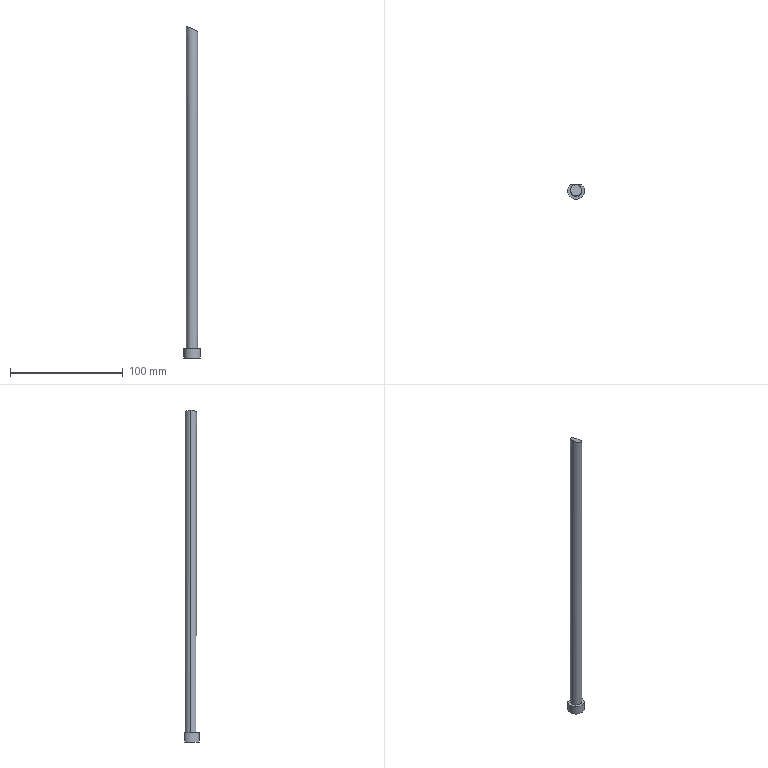Part | Creo | 1 solid | 7 faces | box 15 x 13 x 293.929 mm | volume 23558 mm3 | plane 4 | cylinder 3 | commonest cylinder face diameters 10 x2 15 x1
STEP:
#1=CARTESIAN_POINT('',(0.,0.,0.));
#2=DIRECTION('',(0.,0.,1.));
#3=DIRECTION('',(1.,0.,0.));
#4=AXIS2_PLACEMENT_3D('',#1,#2,#3);
#5=CARTESIAN_POINT('',(124.466,-67.609,-330.441));
#6=VERTEX_POINT('',#5);
#7=CARTESIAN_POINT('',(122.065,-73.109,-330.441));
#8=VERTEX_POINT('',#7);
#9=CARTESIAN_POINT('',(129.565,-73.109,-330.441));
#10=DIRECTION('',(0.,0.,1.));
#11=DIRECTION('',(-0.6799,0.7333,0.));
#12=AXIS2_PLACEMENT_3D('',#9,#10,#11);
#13=CIRCLE('',#12,7.5);
#14=EDGE_CURVE('',#6,#8,#13,.T.);
#15=ORIENTED_EDGE('',*,*,#14,.F.);
#16=CARTESIAN_POINT('',(134.664,-67.609,-330.441));
#17=VERTEX_POINT('',#16);
#18=CARTESIAN_POINT('',(124.466,-67.609,-330.441));
#19=DIRECTION('',(1.,0.,0.));
#20=VECTOR('',#19,10.198);
#21=LINE('',#18,#20);
#22=EDGE_CURVE('',#6,#17,#21,.T.);
#23=ORIENTED_EDGE('',*,*,#22,.T.);
#24=CARTESIAN_POINT('',(129.565,-73.109,-330.441));
#25=DIRECTION('',(0.,0.,1.));
#26=DIRECTION('',(-1.,0.,0.));
#27=AXIS2_PLACEMENT_3D('',#24,#25,#26);
#28=CIRCLE('',#27,7.5);
#29=EDGE_CURVE('',#8,#17,#28,.T.);
#30=ORIENTED_EDGE('',*,*,#29,.F.);
#31=EDGE_LOOP('',(#15,#23,#30));
#32=FACE_OUTER_BOUND('',#31,.F.);
#33=CARTESIAN_POINT('',(134.565,-73.109,-330.441));
#34=VERTEX_POINT('',#33);
#35=CARTESIAN_POINT('',(124.565,-73.109,-330.441));
#36=VERTEX_POINT('',#35);
#37=CARTESIAN_POINT('',(129.565,-73.109,-330.441));
#38=DIRECTION('',(0.,0.,-1.));
#39=DIRECTION('',(1.,0.,0.));
#40=AXIS2_PLACEMENT_3D('',#37,#38,#39);
#41=CIRCLE('',#40,5.);
#42=EDGE_CURVE('',#34,#36,#41,.T.);
#43=ORIENTED_EDGE('',*,*,#42,.F.);
#44=CARTESIAN_POINT('',(129.565,-73.109,-330.441));
#45=DIRECTION('',(0.,0.,-1.));
#46=DIRECTION('',(-1.,0.,0.));
#47=AXIS2_PLACEMENT_3D('',#44,#45,#46);
#48=CIRCLE('',#47,5.);
#49=EDGE_CURVE('',#36,#34,#48,.T.);
#50=ORIENTED_EDGE('',*,*,#49,.F.);
#51=EDGE_LOOP('',(#43,#50));
#52=FACE_BOUND('',#51,.F.);
#53=CARTESIAN_POINT('',(129.565,-73.109,-330.441));
#54=DIRECTION('',(0.,0.,1.));
#55=DIRECTION('',(1.,0.,0.));
#56=AXIS2_PLACEMENT_3D('',#53,#54,#55);
#57=PLANE('',#56);
#58=ADVANCED_FACE('',(#32,#52),#57,.T.);
#59=ORIENTED_EDGE('',*,*,#42,.T.);
#60=CARTESIAN_POINT('',(124.565,-73.109,-44.513));
#61=VERTEX_POINT('',#60);
#62=CARTESIAN_POINT('',(124.565,-73.109,-330.441));
#63=DIRECTION('',(0.,0.,1.));
#64=VECTOR('',#63,285.928);
#65=LINE('',#62,#64);
#66=EDGE_CURVE('',#36,#61,#65,.T.);
#67=ORIENTED_EDGE('',*,*,#66,.T.);
#68=CARTESIAN_POINT('',(134.565,-73.109,-49.307));
#69=VERTEX_POINT('',#68);
#70=CARTESIAN_POINT('',(124.565,-73.109,-44.513));
#71=CARTESIAN_POINT('',(124.565,-73.698,-44.519));
#72=CARTESIAN_POINT('',(124.778,-74.971,-44.635));
#73=CARTESIAN_POINT('',(125.925,-76.75,-45.202));
#74=CARTESIAN_POINT('',(127.404,-77.704,-45.921));
#75=CARTESIAN_POINT('',(128.662,-78.057,-46.528));
#76=CARTESIAN_POINT('',(129.565,-78.135,-46.962));
#77=CARTESIAN_POINT('',(130.468,-78.057,-47.394));
#78=CARTESIAN_POINT('',(131.726,-77.704,-47.993));
#79=CARTESIAN_POINT('',(133.205,-76.75,-48.692));
#80=CARTESIAN_POINT('',(134.352,-74.971,-49.224));
#81=CARTESIAN_POINT('',(134.565,-73.698,-49.313));
#82=CARTESIAN_POINT('',(134.565,-73.109,-49.307));
#83=B_SPLINE_CURVE_WITH_KNOTS('',3,(#70,#71,#72,#73,#74,#75,#76,#77,#78,#79,#80,#81,#82),.UNSPECIFIED.,.F.,.F.,(4,1,1,1,1,1,1,1,1,1,4),(0.,0.125,0.25,0.375,0.4375,0.5,0.5625,0.625,0.75,0.875,1.),.UNSPECIFIED.);
#84=EDGE_CURVE('',#61,#69,#83,.T.);
#85=ORIENTED_EDGE('',*,*,#84,.T.);
#86=CARTESIAN_POINT('',(134.565,-73.109,-330.441));
#87=DIRECTION('',(0.,0.,1.));
#88=VECTOR('',#87,281.135);
#89=LINE('',#86,#88);
#90=EDGE_CURVE('',#34,#69,#89,.T.);
#91=ORIENTED_EDGE('',*,*,#90,.F.);
#92=EDGE_LOOP('',(#59,#67,#85,#91));
#93=FACE_OUTER_BOUND('',#92,.F.);
#94=CARTESIAN_POINT('',(129.565,-73.109,-653.441));
#95=DIRECTION('',(0.,0.,1.));
#96=DIRECTION('',(1.,0.,0.));
#97=AXIS2_PLACEMENT_3D('',#94,#95,#96);
#98=CYLINDRICAL_SURFACE('',#97,5.);
#99=ADVANCED_FACE('',(#93),#98,.T.);
#100=ORIENTED_EDGE('',*,*,#49,.T.);
#101=ORIENTED_EDGE('',*,*,#90,.T.);
#102=CARTESIAN_POINT('',(124.566,-73.002,-44.513));
#103=VERTEX_POINT('',#102);
#104=CARTESIAN_POINT('',(134.565,-73.109,-49.307));
#105=CARTESIAN_POINT('',(134.565,-73.033,-49.306));
#106=CARTESIAN_POINT('',(134.564,-73.001,-49.305));
#107=CARTESIAN_POINT('',(134.561,-72.909,-49.303));
#108=CARTESIAN_POINT('',(134.558,-72.844,-49.301));
#109=CARTESIAN_POINT('',(134.554,-72.774,-49.298));
#110=CARTESIAN_POINT('',(134.548,-72.698,-49.295));
#111=CARTESIAN_POINT('',(134.541,-72.617,-49.29));
#112=CARTESIAN_POINT('',(134.529,-72.507,-49.283));
#113=CARTESIAN_POINT('',(134.514,-72.394,-49.275));
#114=CARTESIAN_POINT('',(134.496,-72.278,-49.265));
#115=CARTESIAN_POINT('',(134.477,-72.175,-49.255));
#116=CARTESIAN_POINT('',(134.452,-72.052,-49.242));
#117=CARTESIAN_POINT('',(134.421,-71.916,-49.226));
#118=CARTESIAN_POINT('',(134.384,-71.773,-49.206));
#119=CARTESIAN_POINT('',(134.346,-71.645,-49.187));
#120=CARTESIAN_POINT('',(134.308,-71.527,-49.168));
#121=CARTESIAN_POINT('',(134.258,-71.381,-49.142));
#122=CARTESIAN_POINT('',(134.194,-71.217,-49.11));
#123=CARTESIAN_POINT('',(134.118,-71.041,-49.072));
#124=CARTESIAN_POINT('',(134.042,-70.881,-49.033));
#125=CARTESIAN_POINT('',(133.94,-70.684,-48.982));
#126=CARTESIAN_POINT('',(133.812,-70.465,-48.919));
#127=CARTESIAN_POINT('',(133.658,-70.234,-48.843));
#128=CARTESIAN_POINT('',(133.504,-70.026,-48.767));
#129=CARTESIAN_POINT('',(133.35,-69.839,-48.691));
#130=CARTESIAN_POINT('',(133.195,-69.669,-48.615));
#131=CARTESIAN_POINT('',(132.989,-69.461,-48.514));
#132=CARTESIAN_POINT('',(132.731,-69.233,-48.388));
#133=CARTESIAN_POINT('',(132.421,-69.,-48.237));
#134=CARTESIAN_POINT('',(132.111,-68.801,-48.086));
#135=CARTESIAN_POINT('',(131.8,-68.632,-47.936));
#136=CARTESIAN_POINT('',(131.386,-68.443,-47.735));
#137=CARTESIAN_POINT('',(130.867,-68.267,-47.484));
#138=CARTESIAN_POINT('',(130.243,-68.142,-47.184));
#139=CARTESIAN_POINT('',(129.618,-68.096,-46.884));
#140=CARTESIAN_POINT('',(128.993,-68.129,-46.585));
#141=CARTESIAN_POINT('',(128.367,-68.241,-46.286));
#142=CARTESIAN_POINT('',(127.844,-68.405,-46.037));
#143=CARTESIAN_POINT('',(127.426,-68.585,-45.838));
#144=CARTESIAN_POINT('',(127.112,-68.747,-45.689));
#145=CARTESIAN_POINT('',(126.797,-68.939,-45.541));
#146=CARTESIAN_POINT('',(126.482,-69.166,-45.392));
#147=CARTESIAN_POINT('',(126.219,-69.389,-45.268));
#148=CARTESIAN_POINT('',(126.009,-69.592,-45.169));
#149=CARTESIAN_POINT('',(125.851,-69.759,-45.095));
#150=CARTESIAN_POINT('',(125.692,-69.943,-45.021));
#151=CARTESIAN_POINT('',(125.534,-70.147,-44.948));
#152=CARTESIAN_POINT('',(125.375,-70.375,-44.874));
#153=CARTESIAN_POINT('',(125.243,-70.591,-44.813));
#154=CARTESIAN_POINT('',(125.137,-70.785,-44.764));
#155=CARTESIAN_POINT('',(125.057,-70.944,-44.727));
#156=CARTESIAN_POINT('',(124.977,-71.118,-44.69));
#157=CARTESIAN_POINT('',(124.91,-71.281,-44.66));
#158=CARTESIAN_POINT('',(124.856,-71.426,-44.636));
#159=CARTESIAN_POINT('',(124.816,-71.543,-44.618));
#160=CARTESIAN_POINT('',(124.776,-71.671,-44.6));
#161=CARTESIAN_POINT('',(124.735,-71.813,-44.582));
#162=CARTESIAN_POINT('',(124.701,-71.948,-44.567));
#163=CARTESIAN_POINT('',(124.674,-72.07,-44.555));
#164=CARTESIAN_POINT('',(124.653,-72.172,-44.546));
#165=CARTESIAN_POINT('',(124.632,-72.288,-44.537));
#166=CARTESIAN_POINT('',(124.615,-72.401,-44.53));
#167=CARTESIAN_POINT('',(124.601,-72.51,-44.524));
#168=CARTESIAN_POINT('',(124.592,-72.591,-44.521));
#169=CARTESIAN_POINT('',(124.584,-72.668,-44.518));
#170=CARTESIAN_POINT('',(124.579,-72.738,-44.516));
#171=CARTESIAN_POINT('',(124.574,-72.802,-44.514));
#172=CARTESIAN_POINT('',(124.57,-72.894,-44.513));
#173=CARTESIAN_POINT('',(124.568,-72.926,-44.513));
#174=B_SPLINE_CURVE_WITH_KNOTS('',3,(#104,#105,#106,#107,#108,#109,#110,#111,#112,#113,#114,#115,#116,#117,#118,#119,#120,#121,#122,#123,#124,#125,#126,#127,#128,#129,#130,#131,#132,#133,#134,#135,#136,#137,#138,#139,#140,#141,#142,#143,#144,#145,#146,#147,#148,#149,#150,#151,#152,#153,#154,#155,#156,#157,#158,#159,#160,#161,#162,#163,#164,#165,#166,#167,#168,#169,#170,#171,#172,#173,#102),.UNSPECIFIED.,.F.,.F.,(4,1,1,1,1,1,1,1,1,1,1,1,1,1,1,1,1,1,1,1,1,1,1,1,1,1,1,1,1,1,1,1,1,1,1,1,1,1,1,1,1,1,1,1,1,1,1,1,1,1,1,1,1,1,1,1,1,1,1,1,1,1,1,1,1,1,1,1,4),(0.,0.0002441,0.0004883,0.0009766,0.001465,0.001953,0.00293,0.003906,0.005859,0.007812,0.009766,0.01172,0.01562,0.01953,0.02344,0.02734,0.03125,0.03906,0.04688,0.05469,0.0625,0.07812,0.09375,0.1094,0.125,0.1406,0.1562,0.1875,0.2188,0.25,0.2812,0.3125,0.375,0.4375,0.5,0.5625,0.625,0.6875,0.7188,0.75,0.7812,0.8125,0.8438,0.8594,0.875,0.8906,0.9062,0.9219,0.9375,0.9453,0.9531,0.9609,0.9688,0.9727,0.9766,0.9805,0.9844,0.9883,0.9902,0.9922,0.9941,0.9961,0.9971,0.998,0.9985,0.999,0.9995,0.9998,1.),.UNSPECIFIED.);
#175=EDGE_CURVE('',#69,#103,#174,.T.);
#176=ORIENTED_EDGE('',*,*,#175,.T.);
#177=CARTESIAN_POINT('',(124.566,-73.002,-44.513));
#178=CARTESIAN_POINT('',(124.565,-73.038,-44.513));
#179=CARTESIAN_POINT('',(124.565,-73.073,-44.513));
#180=CARTESIAN_POINT('',(124.565,-73.109,-44.513));
#181=B_SPLINE_CURVE_WITH_KNOTS('',3,(#177,#178,#179,#180),.UNSPECIFIED.,.F.,.F.,(4,4),(0.,1.),.UNSPECIFIED.);
#182=EDGE_CURVE('',#103,#61,#181,.T.);
#183=ORIENTED_EDGE('',*,*,#182,.T.);
#184=ORIENTED_EDGE('',*,*,#66,.F.);
#185=EDGE_LOOP('',(#100,#101,#176,#183,#184));
#186=FACE_OUTER_BOUND('',#185,.F.);
#187=CARTESIAN_POINT('',(129.565,-73.109,-653.441));
#188=DIRECTION('',(0.,0.,1.));
#189=DIRECTION('',(1.,0.,0.));
#190=AXIS2_PLACEMENT_3D('',#187,#188,#189);
#191=CYLINDRICAL_SURFACE('',#190,5.);
#192=ADVANCED_FACE('',(#186),#191,.T.);
#193=ORIENTED_EDGE('',*,*,#182,.F.);
#194=ORIENTED_EDGE('',*,*,#175,.F.);
#195=ORIENTED_EDGE('',*,*,#84,.F.);
#196=EDGE_LOOP('',(#193,#194,#195));
#197=FACE_OUTER_BOUND('',#196,.F.);
#198=CARTESIAN_POINT('',(120.461,-79.788,-42.615));
#199=DIRECTION('',(-0.4322,0.009245,-0.9017));
#200=DIRECTION('',(-0.9018,0.,0.4323));
#201=AXIS2_PLACEMENT_3D('',#198,#199,#200);
#202=PLANE('',#201);
#203=ADVANCED_FACE('',(#197),#202,.F.);
#204=CARTESIAN_POINT('',(134.664,-67.609,-338.441));
#205=VERTEX_POINT('',#204);
#206=CARTESIAN_POINT('',(134.664,-67.609,-338.441));
#207=DIRECTION('',(0.,0.,1.));
#208=VECTOR('',#207,8.);
#209=LINE('',#206,#208);
#210=EDGE_CURVE('',#205,#17,#209,.T.);
#211=ORIENTED_EDGE('',*,*,#210,.F.);
#212=CARTESIAN_POINT('',(122.065,-73.109,-338.441));
#213=VERTEX_POINT('',#212);
#214=CARTESIAN_POINT('',(129.565,-73.109,-338.441));
#215=DIRECTION('',(0.,0.,-1.));
#216=DIRECTION('',(0.6799,0.7333,0.));
#217=AXIS2_PLACEMENT_3D('',#214,#215,#216);
#218=CIRCLE('',#217,7.5);
#219=EDGE_CURVE('',#205,#213,#218,.T.);
#220=ORIENTED_EDGE('',*,*,#219,.T.);
#221=CARTESIAN_POINT('',(124.466,-67.609,-338.441));
#222=VERTEX_POINT('',#221);
#223=CARTESIAN_POINT('',(129.565,-73.109,-338.441));
#224=DIRECTION('',(0.,0.,-1.));
#225=DIRECTION('',(-1.,0.,0.));
#226=AXIS2_PLACEMENT_3D('',#223,#224,#225);
#227=CIRCLE('',#226,7.5);
#228=EDGE_CURVE('',#213,#222,#227,.T.);
#229=ORIENTED_EDGE('',*,*,#228,.T.);
#230=CARTESIAN_POINT('',(124.466,-67.609,-330.441));
#231=DIRECTION('',(0.,0.,-1.));
#232=VECTOR('',#231,8.);
#233=LINE('',#230,#232);
#234=EDGE_CURVE('',#6,#222,#233,.T.);
#235=ORIENTED_EDGE('',*,*,#234,.F.);
#236=ORIENTED_EDGE('',*,*,#14,.T.);
#237=ORIENTED_EDGE('',*,*,#29,.T.);
#238=EDGE_LOOP('',(#211,#220,#229,#235,#236,#237));
#239=FACE_OUTER_BOUND('',#238,.F.);
#240=CARTESIAN_POINT('',(129.565,-73.109,-330.441));
#241=DIRECTION('',(0.,0.,-1.));
#242=DIRECTION('',(-1.,0.,0.));
#243=AXIS2_PLACEMENT_3D('',#240,#241,#242);
#244=CYLINDRICAL_SURFACE('',#243,7.5);
#245=ADVANCED_FACE('',(#239),#244,.T.);
#246=ORIENTED_EDGE('',*,*,#22,.F.);
#247=ORIENTED_EDGE('',*,*,#234,.T.);
#248=CARTESIAN_POINT('',(124.466,-67.609,-338.441));
#249=DIRECTION('',(1.,0.,0.));
#250=VECTOR('',#249,10.198);
#251=LINE('',#248,#250);
#252=EDGE_CURVE('',#222,#205,#251,.T.);
#253=ORIENTED_EDGE('',*,*,#252,.T.);
#254=ORIENTED_EDGE('',*,*,#210,.T.);
#255=EDGE_LOOP('',(#246,#247,#253,#254));
#256=FACE_OUTER_BOUND('',#255,.F.);
#257=CARTESIAN_POINT('',(129.565,-67.609,-338.441));
#258=DIRECTION('',(0.,1.,0.));
#259=DIRECTION('',(0.,0.,1.));
#260=AXIS2_PLACEMENT_3D('',#257,#258,#259);
#261=PLANE('',#260);
#262=ADVANCED_FACE('',(#256),#261,.T.);
#263=ORIENTED_EDGE('',*,*,#252,.F.);
#264=ORIENTED_EDGE('',*,*,#228,.F.);
#265=ORIENTED_EDGE('',*,*,#219,.F.);
#266=EDGE_LOOP('',(#263,#264,#265));
#267=FACE_OUTER_BOUND('',#266,.F.);
#268=CARTESIAN_POINT('',(129.565,-73.109,-338.441));
#269=DIRECTION('',(0.,0.,1.));
#270=DIRECTION('',(1.,0.,0.));
#271=AXIS2_PLACEMENT_3D('',#268,#269,#270);
#272=PLANE('',#271);
#273=ADVANCED_FACE('',(#267),#272,.F.);
#274=CLOSED_SHELL('',(#58,#99,#192,#203,#245,#262,#273));
#275=MANIFOLD_SOLID_BREP('',#274);
#276=(LENGTH_UNIT()NAMED_UNIT(*)SI_UNIT(.MILLI.,.METRE.));
#277=UNCERTAINTY_MEASURE_WITH_UNIT(LENGTH_MEASURE(0.02946),#276,'','');
#278=(NAMED_UNIT(*)PLANE_ANGLE_UNIT()SI_UNIT($,.RADIAN.));
#279=PLANE_ANGLE_MEASURE_WITH_UNIT(PLANE_ANGLE_MEASURE(0.01745),#278);
#280=(CONVERSION_BASED_UNIT('DEGREE',#279)NAMED_UNIT(*)PLANE_ANGLE_UNIT());
#281=(NAMED_UNIT(*)SI_UNIT($,.STERADIAN.)SOLID_ANGLE_UNIT());
#282=(GEOMETRIC_REPRESENTATION_CONTEXT(3)GLOBAL_UNCERTAINTY_ASSIGNED_CONTEXT((#277))GLOBAL_UNIT_ASSIGNED_CONTEXT((#276,#280,#281))REPRESENTATION_CONTEXT('',''));
#283=ADVANCED_BREP_SHAPE_REPRESENTATION('',(#4,#275),#282);